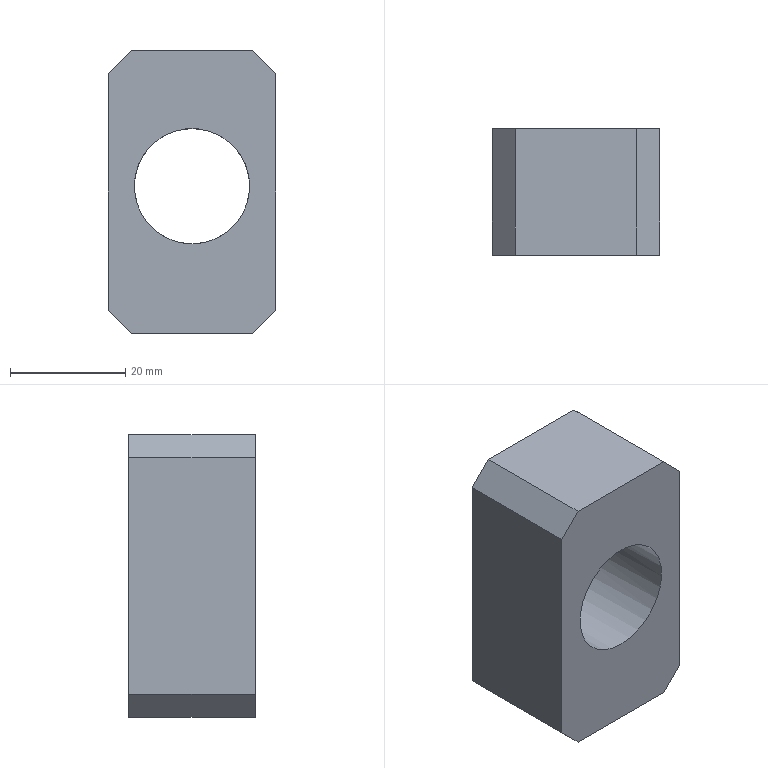Part | NX | features solid 2 | 1 solid | 24 faces | box 29 x 22 x 49 mm | volume 21957 mm3 | plane 14 | cylinder 8 | cone 2 | commonest cylinder face diameters 4 x2 5 x2 6 x2 20 x1 26 x1
STEP:
#1=CARTESIAN_POINT('',(14.5,110.,28.225));
#2=VERTEX_POINT('',#1);
#3=CARTESIAN_POINT('',(14.5,110.,-12.775));
#4=VERTEX_POINT('',#3);
#5=CARTESIAN_POINT('',(14.5,110.,-2.775));
#6=DIRECTION('',(0.,0.,1.));
#7=VECTOR('',#6,1000.);
#8=LINE('',#5,#7);
#9=EDGE_CURVE('',#2,#4,#8,.F.);
#10=ORIENTED_EDGE('',*,*,#9,.F.);
#11=CARTESIAN_POINT('',(10.5,110.,32.225));
#12=VERTEX_POINT('',#11);
#13=CARTESIAN_POINT('',(22.75,110.,19.975));
#14=DIRECTION('',(-0.7071,0.,0.7071));
#15=VECTOR('',#14,1000.);
#16=LINE('',#13,#15);
#17=EDGE_CURVE('',#2,#12,#16,.T.);
#18=ORIENTED_EDGE('',*,*,#17,.T.);
#19=CARTESIAN_POINT('',(-10.5,110.,32.225));
#20=VERTEX_POINT('',#19);
#21=CARTESIAN_POINT('',(0.,110.,32.225));
#22=DIRECTION('',(1.,0.,0.));
#23=VECTOR('',#22,1000.);
#24=LINE('',#21,#23);
#25=EDGE_CURVE('',#12,#20,#24,.F.);
#26=ORIENTED_EDGE('',*,*,#25,.T.);
#27=CARTESIAN_POINT('',(-14.5,110.,28.225));
#28=VERTEX_POINT('',#27);
#29=CARTESIAN_POINT('',(-22.75,110.,19.975));
#30=DIRECTION('',(-0.7071,0.,-0.7071));
#31=VECTOR('',#30,1000.);
#32=LINE('',#29,#31);
#33=EDGE_CURVE('',#20,#28,#32,.T.);
#34=ORIENTED_EDGE('',*,*,#33,.T.);
#35=CARTESIAN_POINT('',(-14.5,110.,-12.775));
#36=VERTEX_POINT('',#35);
#37=CARTESIAN_POINT('',(-14.5,110.,-2.775));
#38=DIRECTION('',(0.,0.,1.));
#39=VECTOR('',#38,1000.);
#40=LINE('',#37,#39);
#41=EDGE_CURVE('',#28,#36,#40,.F.);
#42=ORIENTED_EDGE('',*,*,#41,.T.);
#43=CARTESIAN_POINT('',(-10.5,110.,-16.775));
#44=VERTEX_POINT('',#43);
#45=CARTESIAN_POINT('',(-11.25,110.,-16.025));
#46=DIRECTION('',(0.7071,0.,-0.7071));
#47=VECTOR('',#46,1000.);
#48=LINE('',#45,#47);
#49=EDGE_CURVE('',#36,#44,#48,.T.);
#50=ORIENTED_EDGE('',*,*,#49,.T.);
#51=CARTESIAN_POINT('',(10.5,110.,-16.775));
#52=VERTEX_POINT('',#51);
#53=CARTESIAN_POINT('',(0.,110.,-16.775));
#54=DIRECTION('',(-1.,0.,0.));
#55=VECTOR('',#54,1000.);
#56=LINE('',#53,#55);
#57=EDGE_CURVE('',#44,#52,#56,.F.);
#58=ORIENTED_EDGE('',*,*,#57,.T.);
#59=CARTESIAN_POINT('',(11.25,110.,-16.025));
#60=DIRECTION('',(0.7071,0.,0.7071));
#61=VECTOR('',#60,1000.);
#62=LINE('',#59,#61);
#63=EDGE_CURVE('',#52,#4,#62,.T.);
#64=ORIENTED_EDGE('',*,*,#63,.T.);
#65=EDGE_LOOP('',(#10,#18,#26,#34,#42,#50,#58,#64));
#66=FACE_BOUND('',#65,.T.);
#67=CARTESIAN_POINT('',(0.,110.,-1.275));
#68=VERTEX_POINT('',#67);
#69=CARTESIAN_POINT('',(0.,110.,8.725));
#70=DIRECTION('',(0.,-1.,0.));
#71=DIRECTION('',(0.,0.,-1.));
#72=AXIS2_PLACEMENT_3D('',#69,#70,#71);
#73=CIRCLE('',#72,10.);
#74=EDGE_CURVE('',#68,#68,#73,.T.);
#75=ORIENTED_EDGE('',*,*,#74,.F.);
#76=EDGE_LOOP('',(#75));
#77=FACE_BOUND('',#76,.T.);
#78=CARTESIAN_POINT('',(0.,110.,-2.775));
#79=DIRECTION('',(0.,-1.,0.));
#80=DIRECTION('',(0.,0.,1.));
#81=AXIS2_PLACEMENT_3D('',#78,#79,#80);
#82=PLANE('',#81);
#83=ADVANCED_FACE('',(#66,#77),#82,.T.);
#84=CARTESIAN_POINT('',(-8.923,132.,18.18));
#85=VERTEX_POINT('',#84);
#86=CARTESIAN_POINT('',(8.923,132.,18.18));
#87=VERTEX_POINT('',#86);
#88=CARTESIAN_POINT('',(0.,132.,8.725));
#89=DIRECTION('',(0.,1.,0.));
#90=DIRECTION('',(0.,0.,1.));
#91=AXIS2_PLACEMENT_3D('',#88,#89,#90);
#92=CIRCLE('',#91,13.);
#93=EDGE_CURVE('',#85,#87,#92,.F.);
#94=ORIENTED_EDGE('',*,*,#93,.T.);
#95=CARTESIAN_POINT('',(7.55,132.,18.725));
#96=VERTEX_POINT('',#95);
#97=CARTESIAN_POINT('',(7.55,132.,16.725));
#98=DIRECTION('',(0.,1.,0.));
#99=DIRECTION('',(0.,0.,1.));
#100=AXIS2_PLACEMENT_3D('',#97,#98,#99);
#101=CIRCLE('',#100,2.);
#102=EDGE_CURVE('',#96,#87,#101,.T.);
#103=ORIENTED_EDGE('',*,*,#102,.F.);
#104=CARTESIAN_POINT('',(-7.55,132.,18.725));
#105=VERTEX_POINT('',#104);
#106=CARTESIAN_POINT('',(0.,132.,18.725));
#107=DIRECTION('',(-1.,0.,0.));
#108=VECTOR('',#107,1000.);
#109=LINE('',#106,#108);
#110=EDGE_CURVE('',#105,#96,#109,.F.);
#111=ORIENTED_EDGE('',*,*,#110,.F.);
#112=CARTESIAN_POINT('',(-7.55,132.,16.725));
#113=DIRECTION('',(0.,1.,0.));
#114=DIRECTION('',(0.,0.,1.));
#115=AXIS2_PLACEMENT_3D('',#112,#113,#114);
#116=CIRCLE('',#115,2.);
#117=EDGE_CURVE('',#85,#105,#116,.T.);
#118=ORIENTED_EDGE('',*,*,#117,.F.);
#119=EDGE_LOOP('',(#94,#103,#111,#118));
#120=FACE_BOUND('',#119,.T.);
#121=CARTESIAN_POINT('',(3.,132.,-10.275));
#122=VERTEX_POINT('',#121);
#123=CARTESIAN_POINT('',(0.,132.,-10.275));
#124=DIRECTION('',(0.,-1.,0.));
#125=DIRECTION('',(1.,0.,0.));
#126=AXIS2_PLACEMENT_3D('',#123,#124,#125);
#127=CIRCLE('',#126,3.);
#128=EDGE_CURVE('',#122,#122,#127,.F.);
#129=ORIENTED_EDGE('',*,*,#128,.F.);
#130=EDGE_LOOP('',(#129));
#131=FACE_BOUND('',#130,.T.);
#132=CARTESIAN_POINT('',(3.,132.,25.725));
#133=VERTEX_POINT('',#132);
#134=CARTESIAN_POINT('',(0.,132.,25.725));
#135=DIRECTION('',(0.,1.,0.));
#136=DIRECTION('',(1.,0.,0.));
#137=AXIS2_PLACEMENT_3D('',#134,#135,#136);
#138=CIRCLE('',#137,3.);
#139=EDGE_CURVE('',#133,#133,#138,.F.);
#140=ORIENTED_EDGE('',*,*,#139,.T.);
#141=EDGE_LOOP('',(#140));
#142=FACE_BOUND('',#141,.T.);
#143=CARTESIAN_POINT('',(10.5,132.,-16.775));
#144=VERTEX_POINT('',#143);
#145=CARTESIAN_POINT('',(-10.5,132.,-16.775));
#146=VERTEX_POINT('',#145);
#147=CARTESIAN_POINT('',(0.,132.,-16.775));
#148=DIRECTION('',(1.,0.,0.));
#149=VECTOR('',#148,1000.);
#150=LINE('',#147,#149);
#151=EDGE_CURVE('',#144,#146,#150,.F.);
#152=ORIENTED_EDGE('',*,*,#151,.T.);
#153=CARTESIAN_POINT('',(-14.5,132.,-12.775));
#154=VERTEX_POINT('',#153);
#155=CARTESIAN_POINT('',(-11.25,132.,-16.025));
#156=DIRECTION('',(-0.7071,0.,0.7071));
#157=VECTOR('',#156,1000.);
#158=LINE('',#155,#157);
#159=EDGE_CURVE('',#146,#154,#158,.T.);
#160=ORIENTED_EDGE('',*,*,#159,.T.);
#161=CARTESIAN_POINT('',(-14.5,132.,28.225));
#162=VERTEX_POINT('',#161);
#163=CARTESIAN_POINT('',(-14.5,132.,-2.775));
#164=DIRECTION('',(0.,0.,1.));
#165=VECTOR('',#164,1000.);
#166=LINE('',#163,#165);
#167=EDGE_CURVE('',#162,#154,#166,.F.);
#168=ORIENTED_EDGE('',*,*,#167,.F.);
#169=CARTESIAN_POINT('',(-10.5,132.,32.225));
#170=VERTEX_POINT('',#169);
#171=CARTESIAN_POINT('',(-22.75,132.,19.975));
#172=DIRECTION('',(0.7071,0.,0.7071));
#173=VECTOR('',#172,1000.);
#174=LINE('',#171,#173);
#175=EDGE_CURVE('',#162,#170,#174,.T.);
#176=ORIENTED_EDGE('',*,*,#175,.T.);
#177=CARTESIAN_POINT('',(10.5,132.,32.225));
#178=VERTEX_POINT('',#177);
#179=CARTESIAN_POINT('',(0.,132.,32.225));
#180=DIRECTION('',(-1.,0.,0.));
#181=VECTOR('',#180,1000.);
#182=LINE('',#179,#181);
#183=EDGE_CURVE('',#170,#178,#182,.F.);
#184=ORIENTED_EDGE('',*,*,#183,.T.);
#185=CARTESIAN_POINT('',(14.5,132.,28.225));
#186=VERTEX_POINT('',#185);
#187=CARTESIAN_POINT('',(22.75,132.,19.975));
#188=DIRECTION('',(0.7071,0.,-0.7071));
#189=VECTOR('',#188,1000.);
#190=LINE('',#187,#189);
#191=EDGE_CURVE('',#178,#186,#190,.T.);
#192=ORIENTED_EDGE('',*,*,#191,.T.);
#193=CARTESIAN_POINT('',(14.5,132.,-12.775));
#194=VERTEX_POINT('',#193);
#195=CARTESIAN_POINT('',(14.5,132.,-2.775));
#196=DIRECTION('',(0.,0.,1.));
#197=VECTOR('',#196,1000.);
#198=LINE('',#195,#197);
#199=EDGE_CURVE('',#186,#194,#198,.F.);
#200=ORIENTED_EDGE('',*,*,#199,.T.);
#201=CARTESIAN_POINT('',(11.25,132.,-16.025));
#202=DIRECTION('',(-0.7071,0.,-0.7071));
#203=VECTOR('',#202,1000.);
#204=LINE('',#201,#203);
#205=EDGE_CURVE('',#194,#144,#204,.T.);
#206=ORIENTED_EDGE('',*,*,#205,.T.);
#207=EDGE_LOOP('',(#152,#160,#168,#176,#184,#192,#200,#206));
#208=FACE_BOUND('',#207,.T.);
#209=CARTESIAN_POINT('',(0.,132.,-2.775));
#210=DIRECTION('',(0.,1.,0.));
#211=DIRECTION('',(0.,0.,-1.));
#212=AXIS2_PLACEMENT_3D('',#209,#210,#211);
#213=PLANE('',#212);
#214=ADVANCED_FACE('',(#120,#131,#142,#208),#213,.T.);
#215=ORIENTED_EDGE('',*,*,#25,.F.);
#216=CARTESIAN_POINT('',(10.5,119.,32.225));
#217=DIRECTION('',(0.,-1.,0.));
#218=VECTOR('',#217,1000.);
#219=LINE('',#216,#218);
#220=EDGE_CURVE('',#12,#178,#219,.F.);
#221=ORIENTED_EDGE('',*,*,#220,.T.);
#222=ORIENTED_EDGE('',*,*,#183,.F.);
#223=CARTESIAN_POINT('',(-10.5,119.,32.225));
#224=DIRECTION('',(0.,1.,0.));
#225=VECTOR('',#224,1000.);
#226=LINE('',#223,#225);
#227=EDGE_CURVE('',#170,#20,#226,.F.);
#228=ORIENTED_EDGE('',*,*,#227,.T.);
#229=EDGE_LOOP('',(#215,#221,#222,#228));
#230=FACE_BOUND('',#229,.T.);
#231=CARTESIAN_POINT('',(0.,119.,32.225));
#232=DIRECTION('',(0.,0.,1.));
#233=DIRECTION('',(1.,0.,0.));
#234=AXIS2_PLACEMENT_3D('',#231,#232,#233);
#235=PLANE('',#234);
#236=ADVANCED_FACE('',(#230),#235,.T.);
#237=ORIENTED_EDGE('',*,*,#199,.F.);
#238=CARTESIAN_POINT('',(14.5,119.,28.225));
#239=DIRECTION('',(0.,1.,0.));
#240=VECTOR('',#239,1000.);
#241=LINE('',#238,#240);
#242=EDGE_CURVE('',#186,#2,#241,.F.);
#243=ORIENTED_EDGE('',*,*,#242,.T.);
#244=ORIENTED_EDGE('',*,*,#9,.T.);
#245=CARTESIAN_POINT('',(14.5,119.,-12.775));
#246=DIRECTION('',(0.,-1.,0.));
#247=VECTOR('',#246,1000.);
#248=LINE('',#245,#247);
#249=EDGE_CURVE('',#4,#194,#248,.F.);
#250=ORIENTED_EDGE('',*,*,#249,.T.);
#251=EDGE_LOOP('',(#237,#243,#244,#250));
#252=FACE_BOUND('',#251,.T.);
#253=CARTESIAN_POINT('',(14.5,119.,-2.775));
#254=DIRECTION('',(1.,0.,0.));
#255=DIRECTION('',(0.,0.,-1.));
#256=AXIS2_PLACEMENT_3D('',#253,#254,#255);
#257=PLANE('',#256);
#258=ADVANCED_FACE('',(#252),#257,.T.);
#259=ORIENTED_EDGE('',*,*,#57,.F.);
#260=CARTESIAN_POINT('',(-10.5,119.,-16.775));
#261=DIRECTION('',(0.,-1.,0.));
#262=VECTOR('',#261,1000.);
#263=LINE('',#260,#262);
#264=EDGE_CURVE('',#44,#146,#263,.F.);
#265=ORIENTED_EDGE('',*,*,#264,.T.);
#266=ORIENTED_EDGE('',*,*,#151,.F.);
#267=CARTESIAN_POINT('',(10.5,119.,-16.775));
#268=DIRECTION('',(0.,1.,0.));
#269=VECTOR('',#268,1000.);
#270=LINE('',#267,#269);
#271=EDGE_CURVE('',#144,#52,#270,.F.);
#272=ORIENTED_EDGE('',*,*,#271,.T.);
#273=EDGE_LOOP('',(#259,#265,#266,#272));
#274=FACE_BOUND('',#273,.T.);
#275=CARTESIAN_POINT('',(0.,119.,-16.775));
#276=DIRECTION('',(0.,0.,-1.));
#277=DIRECTION('',(-1.,0.,0.));
#278=AXIS2_PLACEMENT_3D('',#275,#276,#277);
#279=PLANE('',#278);
#280=ADVANCED_FACE('',(#274),#279,.T.);
#281=ORIENTED_EDGE('',*,*,#41,.F.);
#282=CARTESIAN_POINT('',(-14.5,119.,28.225));
#283=DIRECTION('',(0.,-1.,0.));
#284=VECTOR('',#283,1000.);
#285=LINE('',#282,#284);
#286=EDGE_CURVE('',#28,#162,#285,.F.);
#287=ORIENTED_EDGE('',*,*,#286,.T.);
#288=ORIENTED_EDGE('',*,*,#167,.T.);
#289=CARTESIAN_POINT('',(-14.5,119.,-12.775));
#290=DIRECTION('',(0.,1.,0.));
#291=VECTOR('',#290,1000.);
#292=LINE('',#289,#291);
#293=EDGE_CURVE('',#154,#36,#292,.F.);
#294=ORIENTED_EDGE('',*,*,#293,.T.);
#295=EDGE_LOOP('',(#281,#287,#288,#294));
#296=FACE_BOUND('',#295,.T.);
#297=CARTESIAN_POINT('',(-14.5,119.,-2.775));
#298=DIRECTION('',(-1.,0.,0.));
#299=DIRECTION('',(0.,0.,1.));
#300=AXIS2_PLACEMENT_3D('',#297,#298,#299);
#301=PLANE('',#300);
#302=ADVANCED_FACE('',(#296),#301,.T.);
#303=ORIENTED_EDGE('',*,*,#205,.F.);
#304=ORIENTED_EDGE('',*,*,#249,.F.);
#305=ORIENTED_EDGE('',*,*,#63,.F.);
#306=ORIENTED_EDGE('',*,*,#271,.F.);
#307=EDGE_LOOP('',(#303,#304,#305,#306));
#308=FACE_BOUND('',#307,.T.);
#309=CARTESIAN_POINT('',(14.5,119.,-12.775));
#310=DIRECTION('',(-0.7071,0.,0.7071));
#311=DIRECTION('',(0.,-1.,0.));
#312=AXIS2_PLACEMENT_3D('',#309,#310,#311);
#313=PLANE('',#312);
#314=ADVANCED_FACE('',(#308),#313,.F.);
#315=ORIENTED_EDGE('',*,*,#49,.F.);
#316=ORIENTED_EDGE('',*,*,#293,.F.);
#317=ORIENTED_EDGE('',*,*,#159,.F.);
#318=ORIENTED_EDGE('',*,*,#264,.F.);
#319=EDGE_LOOP('',(#315,#316,#317,#318));
#320=FACE_BOUND('',#319,.T.);
#321=CARTESIAN_POINT('',(-14.5,119.,-12.775));
#322=DIRECTION('',(0.7071,0.,0.7071));
#323=DIRECTION('',(0.,1.,0.));
#324=AXIS2_PLACEMENT_3D('',#321,#322,#323);
#325=PLANE('',#324);
#326=ADVANCED_FACE('',(#320),#325,.F.);
#327=ORIENTED_EDGE('',*,*,#175,.F.);
#328=ORIENTED_EDGE('',*,*,#286,.F.);
#329=ORIENTED_EDGE('',*,*,#33,.F.);
#330=ORIENTED_EDGE('',*,*,#227,.F.);
#331=EDGE_LOOP('',(#327,#328,#329,#330));
#332=FACE_BOUND('',#331,.T.);
#333=CARTESIAN_POINT('',(-14.5,119.,28.225));
#334=DIRECTION('',(0.7071,0.,-0.7071));
#335=DIRECTION('',(0.,-1.,0.));
#336=AXIS2_PLACEMENT_3D('',#333,#334,#335);
#337=PLANE('',#336);
#338=ADVANCED_FACE('',(#332),#337,.F.);
#339=ORIENTED_EDGE('',*,*,#17,.F.);
#340=ORIENTED_EDGE('',*,*,#242,.F.);
#341=ORIENTED_EDGE('',*,*,#191,.F.);
#342=ORIENTED_EDGE('',*,*,#220,.F.);
#343=EDGE_LOOP('',(#339,#340,#341,#342));
#344=FACE_BOUND('',#343,.T.);
#345=CARTESIAN_POINT('',(14.5,119.,28.225));
#346=DIRECTION('',(-0.7071,0.,-0.7071));
#347=DIRECTION('',(0.,1.,0.));
#348=AXIS2_PLACEMENT_3D('',#345,#346,#347);
#349=PLANE('',#348);
#350=ADVANCED_FACE('',(#344),#349,.F.);
#351=CARTESIAN_POINT('',(0.,120.,28.225));
#352=VERTEX_POINT('',#351);
#353=CARTESIAN_POINT('',(0.,120.,25.725));
#354=DIRECTION('',(0.,1.,0.));
#355=DIRECTION('',(0.,0.,1.));
#356=AXIS2_PLACEMENT_3D('',#353,#354,#355);
#357=CIRCLE('',#356,2.5);
#358=EDGE_CURVE('',#352,#352,#357,.T.);
#359=ORIENTED_EDGE('',*,*,#358,.F.);
#360=EDGE_LOOP('',(#359));
#361=FACE_BOUND('',#360,.T.);
#362=CARTESIAN_POINT('',(3.,120.,25.725));
#363=VERTEX_POINT('',#362);
#364=CARTESIAN_POINT('',(0.,120.,25.725));
#365=DIRECTION('',(0.,-1.,0.));
#366=DIRECTION('',(1.,0.,0.));
#367=AXIS2_PLACEMENT_3D('',#364,#365,#366);
#368=CIRCLE('',#367,3.);
#369=EDGE_CURVE('',#363,#363,#368,.T.);
#370=ORIENTED_EDGE('',*,*,#369,.F.);
#371=EDGE_LOOP('',(#370));
#372=FACE_BOUND('',#371,.T.);
#373=CARTESIAN_POINT('',(0.,120.,25.725));
#374=DIRECTION('',(0.,-1.,0.));
#375=DIRECTION('',(0.,0.,1.));
#376=AXIS2_PLACEMENT_3D('',#373,#374,#375);
#377=PLANE('',#376);
#378=ADVANCED_FACE('',(#361,#372),#377,.F.);
#379=ORIENTED_EDGE('',*,*,#369,.T.);
#380=EDGE_LOOP('',(#379));
#381=FACE_BOUND('',#380,.T.);
#382=ORIENTED_EDGE('',*,*,#139,.F.);
#383=EDGE_LOOP('',(#382));
#384=FACE_BOUND('',#383,.T.);
#385=CARTESIAN_POINT('',(0.,132.,25.725));
#386=DIRECTION('',(0.,-1.,0.));
#387=DIRECTION('',(1.,0.,0.));
#388=AXIS2_PLACEMENT_3D('',#385,#386,#387);
#389=CYLINDRICAL_SURFACE('',#388,3.);
#390=ADVANCED_FACE('',(#381,#384),#389,.F.);
#391=ORIENTED_EDGE('',*,*,#358,.T.);
#392=EDGE_LOOP('',(#391));
#393=FACE_BOUND('',#392,.T.);
#394=CARTESIAN_POINT('',(2.5,118.,25.725));
#395=VERTEX_POINT('',#394);
#396=CARTESIAN_POINT('',(0.,118.,25.725));
#397=DIRECTION('',(0.,1.,0.));
#398=DIRECTION('',(1.,0.,0.));
#399=AXIS2_PLACEMENT_3D('',#396,#397,#398);
#400=CIRCLE('',#399,2.5);
#401=EDGE_CURVE('',#395,#395,#400,.T.);
#402=ORIENTED_EDGE('',*,*,#401,.F.);
#403=EDGE_LOOP('',(#402));
#404=FACE_BOUND('',#403,.T.);
#405=CARTESIAN_POINT('',(0.,132.,25.725));
#406=DIRECTION('',(0.,-1.,0.));
#407=DIRECTION('',(1.,0.,0.));
#408=AXIS2_PLACEMENT_3D('',#405,#406,#407);
#409=CYLINDRICAL_SURFACE('',#408,2.5);
#410=ADVANCED_FACE('',(#393,#404),#409,.F.);
#411=ORIENTED_EDGE('',*,*,#401,.T.);
#412=EDGE_LOOP('',(#411));
#413=FACE_BOUND('',#412,.T.);
#414=CARTESIAN_POINT('',(0.,116.498,25.725));
#415=VERTEX_POINT('',#414);
#416=VERTEX_LOOP('',#415);
#417=FACE_BOUND('',#416,.T.);
#418=CARTESIAN_POINT('',(0.,116.498,25.725));
#419=DIRECTION('',(0.,1.,0.));
#420=DIRECTION('',(1.,0.,0.));
#421=AXIS2_PLACEMENT_3D('',#418,#419,#420);
#422=CONICAL_SURFACE('',#421,0.,1.03);
#423=ADVANCED_FACE('',(#413,#417),#422,.F.);
#424=CARTESIAN_POINT('',(0.,120.,-12.775));
#425=VERTEX_POINT('',#424);
#426=CARTESIAN_POINT('',(0.,120.,-10.275));
#427=DIRECTION('',(0.,-1.,0.));
#428=DIRECTION('',(0.,0.,-1.));
#429=AXIS2_PLACEMENT_3D('',#426,#427,#428);
#430=CIRCLE('',#429,2.5);
#431=EDGE_CURVE('',#425,#425,#430,.T.);
#432=ORIENTED_EDGE('',*,*,#431,.T.);
#433=EDGE_LOOP('',(#432));
#434=FACE_BOUND('',#433,.T.);
#435=CARTESIAN_POINT('',(3.,120.,-10.275));
#436=VERTEX_POINT('',#435);
#437=CARTESIAN_POINT('',(0.,120.,-10.275));
#438=DIRECTION('',(0.,1.,0.));
#439=DIRECTION('',(1.,0.,0.));
#440=AXIS2_PLACEMENT_3D('',#437,#438,#439);
#441=CIRCLE('',#440,3.);
#442=EDGE_CURVE('',#436,#436,#441,.T.);
#443=ORIENTED_EDGE('',*,*,#442,.T.);
#444=EDGE_LOOP('',(#443));
#445=FACE_BOUND('',#444,.T.);
#446=CARTESIAN_POINT('',(0.,120.,-10.275));
#447=DIRECTION('',(0.,-1.,0.));
#448=DIRECTION('',(0.,0.,-1.));
#449=AXIS2_PLACEMENT_3D('',#446,#447,#448);
#450=PLANE('',#449);
#451=ADVANCED_FACE('',(#434,#445),#450,.F.);
#452=ORIENTED_EDGE('',*,*,#442,.F.);
#453=EDGE_LOOP('',(#452));
#454=FACE_BOUND('',#453,.T.);
#455=ORIENTED_EDGE('',*,*,#128,.T.);
#456=EDGE_LOOP('',(#455));
#457=FACE_BOUND('',#456,.T.);
#458=CARTESIAN_POINT('',(0.,132.,-10.275));
#459=DIRECTION('',(0.,-1.,0.));
#460=DIRECTION('',(1.,0.,0.));
#461=AXIS2_PLACEMENT_3D('',#458,#459,#460);
#462=CYLINDRICAL_SURFACE('',#461,3.);
#463=ADVANCED_FACE('',(#454,#457),#462,.F.);
#464=ORIENTED_EDGE('',*,*,#431,.F.);
#465=EDGE_LOOP('',(#464));
#466=FACE_BOUND('',#465,.T.);
#467=CARTESIAN_POINT('',(2.5,118.,-10.275));
#468=VERTEX_POINT('',#467);
#469=CARTESIAN_POINT('',(0.,118.,-10.275));
#470=DIRECTION('',(0.,-1.,0.));
#471=DIRECTION('',(1.,0.,0.));
#472=AXIS2_PLACEMENT_3D('',#469,#470,#471);
#473=CIRCLE('',#472,2.5);
#474=EDGE_CURVE('',#468,#468,#473,.T.);
#475=ORIENTED_EDGE('',*,*,#474,.T.);
#476=EDGE_LOOP('',(#475));
#477=FACE_BOUND('',#476,.T.);
#478=CARTESIAN_POINT('',(0.,132.,-10.275));
#479=DIRECTION('',(0.,-1.,0.));
#480=DIRECTION('',(1.,0.,0.));
#481=AXIS2_PLACEMENT_3D('',#478,#479,#480);
#482=CYLINDRICAL_SURFACE('',#481,2.5);
#483=ADVANCED_FACE('',(#466,#477),#482,.F.);
#484=ORIENTED_EDGE('',*,*,#474,.F.);
#485=EDGE_LOOP('',(#484));
#486=FACE_BOUND('',#485,.T.);
#487=CARTESIAN_POINT('',(0.,116.498,-10.275));
#488=VERTEX_POINT('',#487);
#489=VERTEX_LOOP('',#488);
#490=FACE_BOUND('',#489,.T.);
#491=CARTESIAN_POINT('',(0.,116.498,-10.275));
#492=DIRECTION('',(0.,1.,0.));
#493=DIRECTION('',(1.,0.,0.));
#494=AXIS2_PLACEMENT_3D('',#491,#492,#493);
#495=CONICAL_SURFACE('',#494,0.,1.03);
#496=ADVANCED_FACE('',(#486,#490),#495,.F.);
#497=ORIENTED_EDGE('',*,*,#74,.T.);
#498=EDGE_LOOP('',(#497));
#499=FACE_BOUND('',#498,.T.);
#500=CARTESIAN_POINT('',(0.,127.,18.725));
#501=VERTEX_POINT('',#500);
#502=CARTESIAN_POINT('',(0.,127.,8.725));
#503=DIRECTION('',(0.,1.,0.));
#504=DIRECTION('',(0.,0.,1.));
#505=AXIS2_PLACEMENT_3D('',#502,#503,#504);
#506=CIRCLE('',#505,10.);
#507=EDGE_CURVE('',#501,#501,#506,.F.);
#508=ORIENTED_EDGE('',*,*,#507,.F.);
#509=EDGE_LOOP('',(#508));
#510=FACE_BOUND('',#509,.T.);
#511=CARTESIAN_POINT('',(0.,125.625,8.725));
#512=DIRECTION('',(0.,-1.,0.));
#513=DIRECTION('',(0.,0.,-1.));
#514=AXIS2_PLACEMENT_3D('',#511,#512,#513);
#515=CYLINDRICAL_SURFACE('',#514,10.);
#516=ADVANCED_FACE('',(#499,#510),#515,.F.);
#517=CARTESIAN_POINT('',(8.923,127.,18.18));
#518=VERTEX_POINT('',#517);
#519=CARTESIAN_POINT('',(-8.923,127.,18.18));
#520=VERTEX_POINT('',#519);
#521=CARTESIAN_POINT('',(0.,127.,8.725));
#522=DIRECTION('',(0.,1.,0.));
#523=DIRECTION('',(0.,0.,1.));
#524=AXIS2_PLACEMENT_3D('',#521,#522,#523);
#525=CIRCLE('',#524,13.);
#526=EDGE_CURVE('',#518,#520,#525,.T.);
#527=ORIENTED_EDGE('',*,*,#526,.T.);
#528=CARTESIAN_POINT('',(-7.55,127.,18.725));
#529=VERTEX_POINT('',#528);
#530=CARTESIAN_POINT('',(-7.55,127.,16.725));
#531=DIRECTION('',(0.,1.,0.));
#532=DIRECTION('',(0.,0.,1.));
#533=AXIS2_PLACEMENT_3D('',#530,#531,#532);
#534=CIRCLE('',#533,2.);
#535=EDGE_CURVE('',#529,#520,#534,.F.);
#536=ORIENTED_EDGE('',*,*,#535,.F.);
#537=CARTESIAN_POINT('',(0.,127.,18.725));
#538=DIRECTION('',(-1.,0.,0.));
#539=VECTOR('',#538,1000.);
#540=LINE('',#537,#539);
#541=EDGE_CURVE('',#529,#501,#540,.F.);
#542=ORIENTED_EDGE('',*,*,#541,.T.);
#543=ORIENTED_EDGE('',*,*,#507,.T.);
#544=CARTESIAN_POINT('',(7.55,127.,18.725));
#545=VERTEX_POINT('',#544);
#546=CARTESIAN_POINT('',(0.,127.,18.725));
#547=DIRECTION('',(-1.,0.,0.));
#548=VECTOR('',#547,1000.);
#549=LINE('',#546,#548);
#550=EDGE_CURVE('',#501,#545,#549,.F.);
#551=ORIENTED_EDGE('',*,*,#550,.T.);
#552=CARTESIAN_POINT('',(7.55,127.,16.725));
#553=DIRECTION('',(0.,1.,0.));
#554=DIRECTION('',(0.,0.,1.));
#555=AXIS2_PLACEMENT_3D('',#552,#553,#554);
#556=CIRCLE('',#555,2.);
#557=EDGE_CURVE('',#518,#545,#556,.F.);
#558=ORIENTED_EDGE('',*,*,#557,.F.);
#559=EDGE_LOOP('',(#527,#536,#542,#543,#551,#558));
#560=FACE_BOUND('',#559,.T.);
#561=CARTESIAN_POINT('',(0.,127.,8.725));
#562=DIRECTION('',(0.,1.,0.));
#563=DIRECTION('',(0.,0.,1.));
#564=AXIS2_PLACEMENT_3D('',#561,#562,#563);
#565=PLANE('',#564);
#566=ADVANCED_FACE('',(#560),#565,.T.);
#567=ORIENTED_EDGE('',*,*,#93,.F.);
#568=CARTESIAN_POINT('',(-8.923,124.,18.18));
#569=DIRECTION('',(0.,1.,0.));
#570=VECTOR('',#569,1000.);
#571=LINE('',#568,#570);
#572=EDGE_CURVE('',#520,#85,#571,.T.);
#573=ORIENTED_EDGE('',*,*,#572,.F.);
#574=ORIENTED_EDGE('',*,*,#526,.F.);
#575=CARTESIAN_POINT('',(8.923,124.,18.18));
#576=DIRECTION('',(0.,1.,0.));
#577=VECTOR('',#576,1000.);
#578=LINE('',#575,#577);
#579=EDGE_CURVE('',#87,#518,#578,.F.);
#580=ORIENTED_EDGE('',*,*,#579,.F.);
#581=EDGE_LOOP('',(#567,#573,#574,#580));
#582=FACE_BOUND('',#581,.T.);
#583=CARTESIAN_POINT('',(0.,124.,8.725));
#584=DIRECTION('',(0.,1.,0.));
#585=DIRECTION('',(0.,0.,1.));
#586=AXIS2_PLACEMENT_3D('',#583,#584,#585);
#587=CYLINDRICAL_SURFACE('',#586,13.);
#588=ADVANCED_FACE('',(#582),#587,.F.);
#589=ORIENTED_EDGE('',*,*,#541,.F.);
#590=CARTESIAN_POINT('',(-7.55,127.,18.725));
#591=DIRECTION('',(0.,1.,0.));
#592=VECTOR('',#591,1000.);
#593=LINE('',#590,#592);
#594=EDGE_CURVE('',#105,#529,#593,.F.);
#595=ORIENTED_EDGE('',*,*,#594,.F.);
#596=ORIENTED_EDGE('',*,*,#110,.T.);
#597=CARTESIAN_POINT('',(7.55,127.,18.725));
#598=DIRECTION('',(0.,1.,0.));
#599=VECTOR('',#598,1000.);
#600=LINE('',#597,#599);
#601=EDGE_CURVE('',#545,#96,#600,.T.);
#602=ORIENTED_EDGE('',*,*,#601,.F.);
#603=ORIENTED_EDGE('',*,*,#550,.F.);
#604=EDGE_LOOP('',(#589,#595,#596,#602,#603));
#605=FACE_BOUND('',#604,.T.);
#606=CARTESIAN_POINT('',(0.,127.,18.725));
#607=DIRECTION('',(0.,0.,-1.));
#608=DIRECTION('',(0.,1.,0.));
#609=AXIS2_PLACEMENT_3D('',#606,#607,#608);
#610=PLANE('',#609);
#611=ADVANCED_FACE('',(#605),#610,.T.);
#612=ORIENTED_EDGE('',*,*,#117,.T.);
#613=ORIENTED_EDGE('',*,*,#594,.T.);
#614=ORIENTED_EDGE('',*,*,#535,.T.);
#615=ORIENTED_EDGE('',*,*,#572,.T.);
#616=EDGE_LOOP('',(#612,#613,#614,#615));
#617=FACE_BOUND('',#616,.T.);
#618=CARTESIAN_POINT('',(-7.55,124.,16.725));
#619=DIRECTION('',(0.,1.,0.));
#620=DIRECTION('',(0.,0.,1.));
#621=AXIS2_PLACEMENT_3D('',#618,#619,#620);
#622=CYLINDRICAL_SURFACE('',#621,2.);
#623=ADVANCED_FACE('',(#617),#622,.F.);
#624=ORIENTED_EDGE('',*,*,#557,.T.);
#625=ORIENTED_EDGE('',*,*,#601,.T.);
#626=ORIENTED_EDGE('',*,*,#102,.T.);
#627=ORIENTED_EDGE('',*,*,#579,.T.);
#628=EDGE_LOOP('',(#624,#625,#626,#627));
#629=FACE_BOUND('',#628,.T.);
#630=CARTESIAN_POINT('',(7.55,124.,16.725));
#631=DIRECTION('',(0.,1.,0.));
#632=DIRECTION('',(0.,0.,1.));
#633=AXIS2_PLACEMENT_3D('',#630,#631,#632);
#634=CYLINDRICAL_SURFACE('',#633,2.);
#635=ADVANCED_FACE('',(#629),#634,.F.);
#636=CLOSED_SHELL('',(#83,#214,#236,#258,#280,#302,#314,#326,#338,#350,#378,#390,#410,#423,#451,#463,#483,#496,#516,#566,#588,#611,#623,#635));
#637=MANIFOLD_SOLID_BREP('',#636);
#638=(LENGTH_UNIT()NAMED_UNIT(*)SI_UNIT(.MILLI.,.METRE.));
#639=UNCERTAINTY_MEASURE_WITH_UNIT(LENGTH_MEASURE(0.00001),#638,'','');
#640=(NAMED_UNIT(*)PLANE_ANGLE_UNIT()SI_UNIT($,.RADIAN.));
#641=(NAMED_UNIT(*)SI_UNIT($,.STERADIAN.)SOLID_ANGLE_UNIT());
#642=(GEOMETRIC_REPRESENTATION_CONTEXT(3)GLOBAL_UNCERTAINTY_ASSIGNED_CONTEXT((#639))GLOBAL_UNIT_ASSIGNED_CONTEXT((#638,#640,#641))REPRESENTATION_CONTEXT('',''));
#643=ADVANCED_BREP_SHAPE_REPRESENTATION('',(#637),#642);